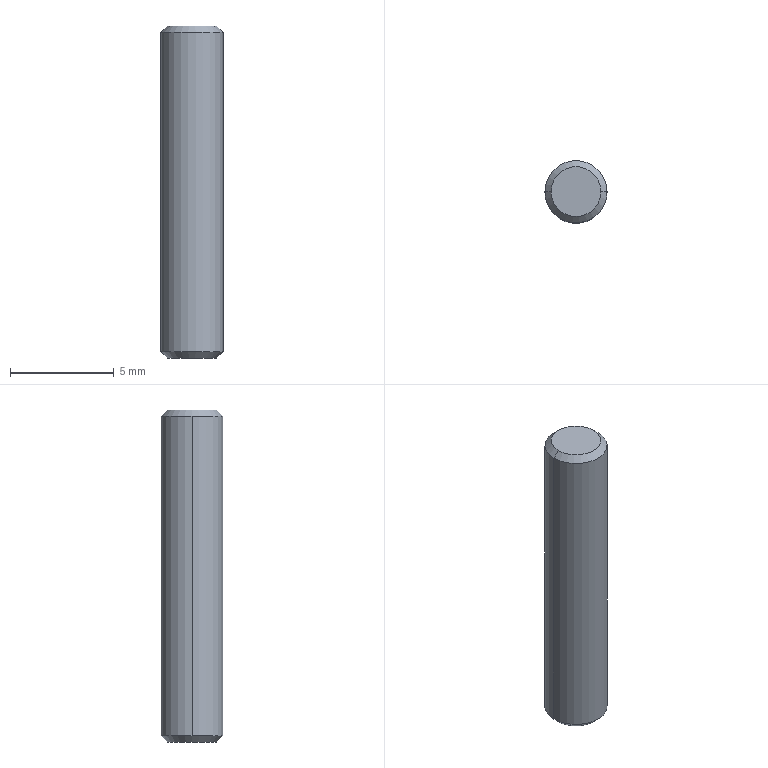Part | NX | features BREP 1 | 1 solid | 8 faces | box 3 x 3 x 16 mm | volume 112.306 mm3 | cone 4 | cylinder 2 | plane 2 | commonest cylinder face diameters 3 x2
STEP:
#1=CARTESIAN_POINT('',(-1.2,0.,-8.));
#2=VERTEX_POINT('',#1);
#3=CARTESIAN_POINT('',(1.2,0.,-8.));
#4=VERTEX_POINT('',#3);
#5=CARTESIAN_POINT('',(0.,0.,-8.));
#6=DIRECTION('',(0.,0.,-1.));
#7=DIRECTION('',(1.,0.,0.));
#8=AXIS2_PLACEMENT_3D('',#5,#6,#7);
#9=CIRCLE('',#8,1.2);
#10=EDGE_CURVE('',#2,#4,#9,.T.);
#11=ORIENTED_EDGE('',*,*,#10,.F.);
#12=CARTESIAN_POINT('',(-1.5,0.,-7.7));
#13=VERTEX_POINT('',#12);
#14=CARTESIAN_POINT('',(-1.5,0.,-7.7));
#15=DIRECTION('',(-0.7071,0.,0.7071));
#16=VECTOR('',#15,1000.);
#17=LINE('',#14,#16);
#18=EDGE_CURVE('',#13,#2,#17,.F.);
#19=ORIENTED_EDGE('',*,*,#18,.F.);
#20=CARTESIAN_POINT('',(1.5,0.,-7.7));
#21=VERTEX_POINT('',#20);
#22=CARTESIAN_POINT('',(0.,0.,-7.7));
#23=DIRECTION('',(0.,0.,1.));
#24=DIRECTION('',(1.,0.,0.));
#25=AXIS2_PLACEMENT_3D('',#22,#23,#24);
#26=CIRCLE('',#25,1.5);
#27=EDGE_CURVE('',#21,#13,#26,.T.);
#28=ORIENTED_EDGE('',*,*,#27,.F.);
#29=CARTESIAN_POINT('',(1.5,0.,-7.7));
#30=DIRECTION('',(0.7071,0.,0.7071));
#31=VECTOR('',#30,1000.);
#32=LINE('',#29,#31);
#33=EDGE_CURVE('',#21,#4,#32,.F.);
#34=ORIENTED_EDGE('',*,*,#33,.T.);
#35=EDGE_LOOP('',(#11,#19,#28,#34));
#36=FACE_BOUND('',#35,.T.);
#37=CARTESIAN_POINT('',(0.,0.,-7.7));
#38=DIRECTION('',(0.,0.,1.));
#39=DIRECTION('',(1.,0.,0.));
#40=AXIS2_PLACEMENT_3D('',#37,#38,#39);
#41=CONICAL_SURFACE('',#40,1.5,0.7854);
#42=ADVANCED_FACE('',(#36),#41,.T.);
#43=CARTESIAN_POINT('',(1.2,0.,8.));
#44=VERTEX_POINT('',#43);
#45=CARTESIAN_POINT('',(-1.2,0.,8.));
#46=VERTEX_POINT('',#45);
#47=CARTESIAN_POINT('',(0.,0.,8.));
#48=DIRECTION('',(0.,0.,1.));
#49=DIRECTION('',(1.,0.,0.));
#50=AXIS2_PLACEMENT_3D('',#47,#48,#49);
#51=CIRCLE('',#50,1.2);
#52=EDGE_CURVE('',#44,#46,#51,.T.);
#53=ORIENTED_EDGE('',*,*,#52,.F.);
#54=CARTESIAN_POINT('',(1.5,0.,7.7));
#55=VERTEX_POINT('',#54);
#56=CARTESIAN_POINT('',(1.2,0.,8.));
#57=DIRECTION('',(0.7071,0.,-0.7071));
#58=VECTOR('',#57,1000.);
#59=LINE('',#56,#58);
#60=EDGE_CURVE('',#44,#55,#59,.T.);
#61=ORIENTED_EDGE('',*,*,#60,.T.);
#62=CARTESIAN_POINT('',(-1.5,0.,7.7));
#63=VERTEX_POINT('',#62);
#64=CARTESIAN_POINT('',(0.,0.,7.7));
#65=DIRECTION('',(0.,0.,-1.));
#66=DIRECTION('',(1.,0.,0.));
#67=AXIS2_PLACEMENT_3D('',#64,#65,#66);
#68=CIRCLE('',#67,1.5);
#69=EDGE_CURVE('',#63,#55,#68,.T.);
#70=ORIENTED_EDGE('',*,*,#69,.F.);
#71=CARTESIAN_POINT('',(-1.2,0.,8.));
#72=DIRECTION('',(-0.7071,0.,-0.7071));
#73=VECTOR('',#72,1000.);
#74=LINE('',#71,#73);
#75=EDGE_CURVE('',#46,#63,#74,.T.);
#76=ORIENTED_EDGE('',*,*,#75,.F.);
#77=EDGE_LOOP('',(#53,#61,#70,#76));
#78=FACE_BOUND('',#77,.T.);
#79=CARTESIAN_POINT('',(0.,0.,8.));
#80=DIRECTION('',(0.,0.,-1.));
#81=DIRECTION('',(-1.,0.,0.));
#82=AXIS2_PLACEMENT_3D('',#79,#80,#81);
#83=CONICAL_SURFACE('',#82,1.2,0.7854);
#84=ADVANCED_FACE('',(#78),#83,.T.);
#85=ORIENTED_EDGE('',*,*,#69,.T.);
#86=CARTESIAN_POINT('',(1.5,0.,8.));
#87=DIRECTION('',(0.,0.,-1.));
#88=VECTOR('',#87,1000.);
#89=LINE('',#86,#88);
#90=EDGE_CURVE('',#55,#21,#89,.T.);
#91=ORIENTED_EDGE('',*,*,#90,.T.);
#92=ORIENTED_EDGE('',*,*,#27,.T.);
#93=CARTESIAN_POINT('',(-1.5,0.,8.));
#94=DIRECTION('',(0.,0.,-1.));
#95=VECTOR('',#94,1000.);
#96=LINE('',#93,#95);
#97=EDGE_CURVE('',#63,#13,#96,.T.);
#98=ORIENTED_EDGE('',*,*,#97,.F.);
#99=EDGE_LOOP('',(#85,#91,#92,#98));
#100=FACE_BOUND('',#99,.T.);
#101=CARTESIAN_POINT('',(0.,0.,8.));
#102=DIRECTION('',(0.,0.,-1.));
#103=DIRECTION('',(-1.,0.,0.));
#104=AXIS2_PLACEMENT_3D('',#101,#102,#103);
#105=CYLINDRICAL_SURFACE('',#104,1.5);
#106=ADVANCED_FACE('',(#100),#105,.T.);
#107=ORIENTED_EDGE('',*,*,#90,.F.);
#108=CARTESIAN_POINT('',(0.,0.,7.7));
#109=DIRECTION('',(0.,0.,-1.));
#110=DIRECTION('',(1.,0.,0.));
#111=AXIS2_PLACEMENT_3D('',#108,#109,#110);
#112=CIRCLE('',#111,1.5);
#113=EDGE_CURVE('',#55,#63,#112,.T.);
#114=ORIENTED_EDGE('',*,*,#113,.T.);
#115=ORIENTED_EDGE('',*,*,#97,.T.);
#116=CARTESIAN_POINT('',(0.,0.,-7.7));
#117=DIRECTION('',(0.,0.,1.));
#118=DIRECTION('',(1.,0.,0.));
#119=AXIS2_PLACEMENT_3D('',#116,#117,#118);
#120=CIRCLE('',#119,1.5);
#121=EDGE_CURVE('',#13,#21,#120,.T.);
#122=ORIENTED_EDGE('',*,*,#121,.T.);
#123=EDGE_LOOP('',(#107,#114,#115,#122));
#124=FACE_BOUND('',#123,.T.);
#125=CARTESIAN_POINT('',(0.,0.,8.));
#126=DIRECTION('',(0.,0.,-1.));
#127=DIRECTION('',(-1.,0.,0.));
#128=AXIS2_PLACEMENT_3D('',#125,#126,#127);
#129=CYLINDRICAL_SURFACE('',#128,1.5);
#130=ADVANCED_FACE('',(#124),#129,.T.);
#131=CARTESIAN_POINT('',(0.,0.,8.));
#132=DIRECTION('',(0.,0.,1.));
#133=DIRECTION('',(1.,0.,0.));
#134=AXIS2_PLACEMENT_3D('',#131,#132,#133);
#135=CIRCLE('',#134,1.2);
#136=EDGE_CURVE('',#46,#44,#135,.T.);
#137=ORIENTED_EDGE('',*,*,#136,.T.);
#138=ORIENTED_EDGE('',*,*,#52,.T.);
#139=EDGE_LOOP('',(#137,#138));
#140=FACE_BOUND('',#139,.T.);
#141=CARTESIAN_POINT('',(0.,0.,8.));
#142=DIRECTION('',(0.,0.,1.));
#143=DIRECTION('',(1.,0.,0.));
#144=AXIS2_PLACEMENT_3D('',#141,#142,#143);
#145=PLANE('',#144);
#146=ADVANCED_FACE('',(#140),#145,.T.);
#147=CARTESIAN_POINT('',(0.,0.,-8.));
#148=DIRECTION('',(0.,0.,-1.));
#149=DIRECTION('',(1.,0.,0.));
#150=AXIS2_PLACEMENT_3D('',#147,#148,#149);
#151=CIRCLE('',#150,1.2);
#152=EDGE_CURVE('',#4,#2,#151,.T.);
#153=ORIENTED_EDGE('',*,*,#152,.T.);
#154=ORIENTED_EDGE('',*,*,#10,.T.);
#155=EDGE_LOOP('',(#153,#154));
#156=FACE_BOUND('',#155,.T.);
#157=CARTESIAN_POINT('',(0.,0.,-8.));
#158=DIRECTION('',(0.,0.,1.));
#159=DIRECTION('',(1.,0.,0.));
#160=AXIS2_PLACEMENT_3D('',#157,#158,#159);
#161=PLANE('',#160);
#162=ADVANCED_FACE('',(#156),#161,.F.);
#163=ORIENTED_EDGE('',*,*,#60,.F.);
#164=ORIENTED_EDGE('',*,*,#136,.F.);
#165=ORIENTED_EDGE('',*,*,#75,.T.);
#166=ORIENTED_EDGE('',*,*,#113,.F.);
#167=EDGE_LOOP('',(#163,#164,#165,#166));
#168=FACE_BOUND('',#167,.T.);
#169=CARTESIAN_POINT('',(0.,0.,8.));
#170=DIRECTION('',(0.,0.,-1.));
#171=DIRECTION('',(-1.,0.,0.));
#172=AXIS2_PLACEMENT_3D('',#169,#170,#171);
#173=CONICAL_SURFACE('',#172,1.2,0.7854);
#174=ADVANCED_FACE('',(#168),#173,.T.);
#175=ORIENTED_EDGE('',*,*,#18,.T.);
#176=ORIENTED_EDGE('',*,*,#152,.F.);
#177=ORIENTED_EDGE('',*,*,#33,.F.);
#178=ORIENTED_EDGE('',*,*,#121,.F.);
#179=EDGE_LOOP('',(#175,#176,#177,#178));
#180=FACE_BOUND('',#179,.T.);
#181=CARTESIAN_POINT('',(0.,0.,-7.7));
#182=DIRECTION('',(0.,0.,1.));
#183=DIRECTION('',(1.,0.,0.));
#184=AXIS2_PLACEMENT_3D('',#181,#182,#183);
#185=CONICAL_SURFACE('',#184,1.5,0.7854);
#186=ADVANCED_FACE('',(#180),#185,.T.);
#187=CLOSED_SHELL('',(#42,#84,#106,#130,#146,#162,#174,#186));
#188=MANIFOLD_SOLID_BREP('',#187);
#189=(LENGTH_UNIT()NAMED_UNIT(*)SI_UNIT(.MILLI.,.METRE.));
#190=UNCERTAINTY_MEASURE_WITH_UNIT(LENGTH_MEASURE(0.00001),#189,'','');
#191=(NAMED_UNIT(*)PLANE_ANGLE_UNIT()SI_UNIT($,.RADIAN.));
#192=(NAMED_UNIT(*)SI_UNIT($,.STERADIAN.)SOLID_ANGLE_UNIT());
#193=(GEOMETRIC_REPRESENTATION_CONTEXT(3)GLOBAL_UNCERTAINTY_ASSIGNED_CONTEXT((#190))GLOBAL_UNIT_ASSIGNED_CONTEXT((#189,#191,#192))REPRESENTATION_CONTEXT('',''));
#194=ADVANCED_BREP_SHAPE_REPRESENTATION('',(#188),#193);